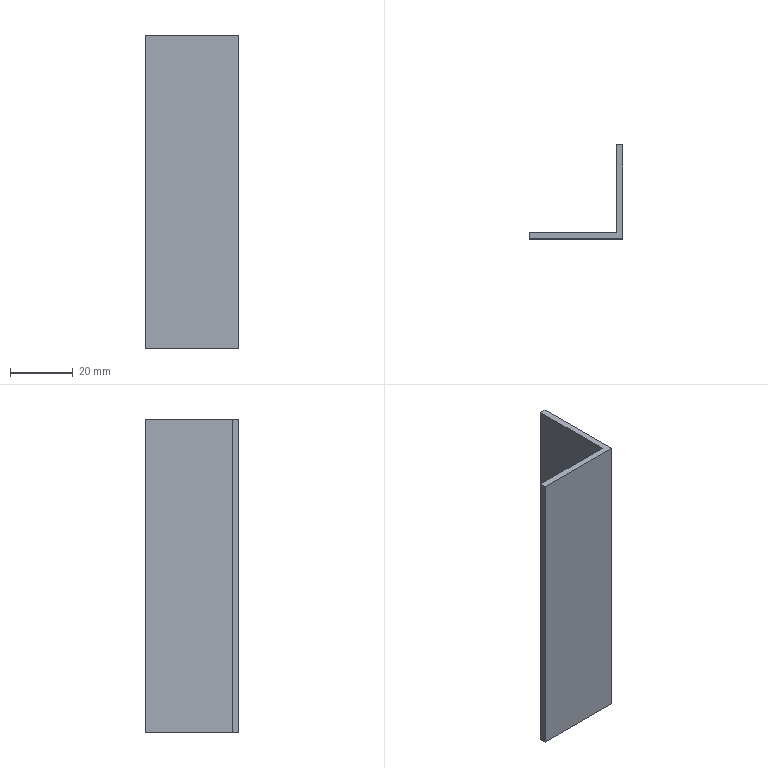Part | SolidWorks | features Extrusion 1 | 1 solid | 8 faces | box 30 x 30 x 100 mm | volume 11600 mm3 | plane 8
STEP:
#1=CARTESIAN_POINT('',(0.,2.,0.));
#2=VERTEX_POINT('',#1);
#3=CARTESIAN_POINT('',(0.,0.,0.));
#4=VERTEX_POINT('',#3);
#5=CARTESIAN_POINT('',(0.,0.,0.));
#6=DIRECTION('',(0.,-1.,0.));
#7=VECTOR('',#6,1000.);
#8=LINE('',#5,#7);
#9=EDGE_CURVE('',#2,#4,#8,.T.);
#10=ORIENTED_EDGE('',*,*,#9,.T.);
#11=CARTESIAN_POINT('',(0.,0.,100.));
#12=VERTEX_POINT('',#11);
#13=CARTESIAN_POINT('',(0.,0.,100.));
#14=DIRECTION('',(0.,0.,-1.));
#15=VECTOR('',#14,1000.);
#16=LINE('',#13,#15);
#17=EDGE_CURVE('',#12,#4,#16,.T.);
#18=ORIENTED_EDGE('',*,*,#17,.F.);
#19=CARTESIAN_POINT('',(0.,2.,100.));
#20=VERTEX_POINT('',#19);
#21=CARTESIAN_POINT('',(0.,0.,100.));
#22=DIRECTION('',(0.,-1.,0.));
#23=VECTOR('',#22,1000.);
#24=LINE('',#21,#23);
#25=EDGE_CURVE('',#20,#12,#24,.T.);
#26=ORIENTED_EDGE('',*,*,#25,.F.);
#27=CARTESIAN_POINT('',(0.,2.,100.));
#28=DIRECTION('',(0.,0.,-1.));
#29=VECTOR('',#28,1000.);
#30=LINE('',#27,#29);
#31=EDGE_CURVE('',#20,#2,#30,.T.);
#32=ORIENTED_EDGE('',*,*,#31,.T.);
#33=EDGE_LOOP('',(#10,#18,#26,#32));
#34=FACE_OUTER_BOUND('',#33,.T.);
#35=CARTESIAN_POINT('',(0.,0.,100.));
#36=DIRECTION('',(1.,0.,0.));
#37=DIRECTION('',(0.,0.,-1.));
#38=AXIS2_PLACEMENT_3D('',#35,#36,#37);
#39=PLANE('',#38);
#40=ADVANCED_FACE('',(#34),#39,.F.);
#41=CARTESIAN_POINT('',(30.,0.,0.));
#42=VERTEX_POINT('',#41);
#43=CARTESIAN_POINT('',(0.,0.,0.));
#44=DIRECTION('',(1.,0.,0.));
#45=VECTOR('',#44,1000.);
#46=LINE('',#43,#45);
#47=EDGE_CURVE('',#4,#42,#46,.T.);
#48=ORIENTED_EDGE('',*,*,#47,.T.);
#49=CARTESIAN_POINT('',(30.,0.,100.));
#50=VERTEX_POINT('',#49);
#51=CARTESIAN_POINT('',(30.,0.,100.));
#52=DIRECTION('',(0.,0.,-1.));
#53=VECTOR('',#52,1000.);
#54=LINE('',#51,#53);
#55=EDGE_CURVE('',#50,#42,#54,.T.);
#56=ORIENTED_EDGE('',*,*,#55,.F.);
#57=CARTESIAN_POINT('',(0.,0.,100.));
#58=DIRECTION('',(1.,0.,0.));
#59=VECTOR('',#58,1000.);
#60=LINE('',#57,#59);
#61=EDGE_CURVE('',#12,#50,#60,.T.);
#62=ORIENTED_EDGE('',*,*,#61,.F.);
#63=ORIENTED_EDGE('',*,*,#17,.T.);
#64=EDGE_LOOP('',(#48,#56,#62,#63));
#65=FACE_OUTER_BOUND('',#64,.T.);
#66=CARTESIAN_POINT('',(0.,0.,100.));
#67=DIRECTION('',(0.,1.,0.));
#68=DIRECTION('',(0.,0.,1.));
#69=AXIS2_PLACEMENT_3D('',#66,#67,#68);
#70=PLANE('',#69);
#71=ADVANCED_FACE('',(#65),#70,.F.);
#72=CARTESIAN_POINT('',(30.,30.,0.));
#73=VERTEX_POINT('',#72);
#74=CARTESIAN_POINT('',(30.,0.,0.));
#75=DIRECTION('',(0.,1.,0.));
#76=VECTOR('',#75,1000.);
#77=LINE('',#74,#76);
#78=EDGE_CURVE('',#42,#73,#77,.T.);
#79=ORIENTED_EDGE('',*,*,#78,.T.);
#80=CARTESIAN_POINT('',(30.,30.,100.));
#81=VERTEX_POINT('',#80);
#82=CARTESIAN_POINT('',(30.,30.,100.));
#83=DIRECTION('',(0.,0.,-1.));
#84=VECTOR('',#83,1000.);
#85=LINE('',#82,#84);
#86=EDGE_CURVE('',#81,#73,#85,.T.);
#87=ORIENTED_EDGE('',*,*,#86,.F.);
#88=CARTESIAN_POINT('',(30.,0.,100.));
#89=DIRECTION('',(0.,1.,0.));
#90=VECTOR('',#89,1000.);
#91=LINE('',#88,#90);
#92=EDGE_CURVE('',#50,#81,#91,.T.);
#93=ORIENTED_EDGE('',*,*,#92,.F.);
#94=ORIENTED_EDGE('',*,*,#55,.T.);
#95=EDGE_LOOP('',(#79,#87,#93,#94));
#96=FACE_OUTER_BOUND('',#95,.T.);
#97=CARTESIAN_POINT('',(30.,0.,100.));
#98=DIRECTION('',(-1.,0.,0.));
#99=DIRECTION('',(0.,0.,1.));
#100=AXIS2_PLACEMENT_3D('',#97,#98,#99);
#101=PLANE('',#100);
#102=ADVANCED_FACE('',(#96),#101,.F.);
#103=CARTESIAN_POINT('',(28.,30.,0.));
#104=VERTEX_POINT('',#103);
#105=CARTESIAN_POINT('',(28.,30.,0.));
#106=DIRECTION('',(-1.,0.,0.));
#107=VECTOR('',#106,1000.);
#108=LINE('',#105,#107);
#109=EDGE_CURVE('',#73,#104,#108,.T.);
#110=ORIENTED_EDGE('',*,*,#109,.T.);
#111=CARTESIAN_POINT('',(28.,30.,100.));
#112=VERTEX_POINT('',#111);
#113=CARTESIAN_POINT('',(28.,30.,100.));
#114=DIRECTION('',(0.,0.,-1.));
#115=VECTOR('',#114,1000.);
#116=LINE('',#113,#115);
#117=EDGE_CURVE('',#112,#104,#116,.T.);
#118=ORIENTED_EDGE('',*,*,#117,.F.);
#119=CARTESIAN_POINT('',(28.,30.,100.));
#120=DIRECTION('',(-1.,0.,0.));
#121=VECTOR('',#120,1000.);
#122=LINE('',#119,#121);
#123=EDGE_CURVE('',#81,#112,#122,.T.);
#124=ORIENTED_EDGE('',*,*,#123,.F.);
#125=ORIENTED_EDGE('',*,*,#86,.T.);
#126=EDGE_LOOP('',(#110,#118,#124,#125));
#127=FACE_OUTER_BOUND('',#126,.T.);
#128=CARTESIAN_POINT('',(28.,30.,100.));
#129=DIRECTION('',(0.,-1.,0.));
#130=DIRECTION('',(0.,0.,-1.));
#131=AXIS2_PLACEMENT_3D('',#128,#129,#130);
#132=PLANE('',#131);
#133=ADVANCED_FACE('',(#127),#132,.F.);
#134=CARTESIAN_POINT('',(28.,2.,0.));
#135=VERTEX_POINT('',#134);
#136=CARTESIAN_POINT('',(28.,2.,0.));
#137=DIRECTION('',(0.,-1.,0.));
#138=VECTOR('',#137,1000.);
#139=LINE('',#136,#138);
#140=EDGE_CURVE('',#104,#135,#139,.T.);
#141=ORIENTED_EDGE('',*,*,#140,.T.);
#142=CARTESIAN_POINT('',(28.,2.,100.));
#143=VERTEX_POINT('',#142);
#144=CARTESIAN_POINT('',(28.,2.,100.));
#145=DIRECTION('',(0.,0.,-1.));
#146=VECTOR('',#145,1000.);
#147=LINE('',#144,#146);
#148=EDGE_CURVE('',#143,#135,#147,.T.);
#149=ORIENTED_EDGE('',*,*,#148,.F.);
#150=CARTESIAN_POINT('',(28.,2.,100.));
#151=DIRECTION('',(0.,-1.,0.));
#152=VECTOR('',#151,1000.);
#153=LINE('',#150,#152);
#154=EDGE_CURVE('',#112,#143,#153,.T.);
#155=ORIENTED_EDGE('',*,*,#154,.F.);
#156=ORIENTED_EDGE('',*,*,#117,.T.);
#157=EDGE_LOOP('',(#141,#149,#155,#156));
#158=FACE_OUTER_BOUND('',#157,.T.);
#159=CARTESIAN_POINT('',(28.,2.,100.));
#160=DIRECTION('',(1.,0.,0.));
#161=DIRECTION('',(0.,0.,-1.));
#162=AXIS2_PLACEMENT_3D('',#159,#160,#161);
#163=PLANE('',#162);
#164=ADVANCED_FACE('',(#158),#163,.F.);
#165=CARTESIAN_POINT('',(0.,2.,0.));
#166=DIRECTION('',(-1.,0.,0.));
#167=VECTOR('',#166,1000.);
#168=LINE('',#165,#167);
#169=EDGE_CURVE('',#135,#2,#168,.T.);
#170=ORIENTED_EDGE('',*,*,#169,.T.);
#171=ORIENTED_EDGE('',*,*,#31,.F.);
#172=CARTESIAN_POINT('',(0.,2.,100.));
#173=DIRECTION('',(-1.,0.,0.));
#174=VECTOR('',#173,1000.);
#175=LINE('',#172,#174);
#176=EDGE_CURVE('',#143,#20,#175,.T.);
#177=ORIENTED_EDGE('',*,*,#176,.F.);
#178=ORIENTED_EDGE('',*,*,#148,.T.);
#179=EDGE_LOOP('',(#170,#171,#177,#178));
#180=FACE_OUTER_BOUND('',#179,.T.);
#181=CARTESIAN_POINT('',(0.,2.,100.));
#182=DIRECTION('',(0.,-1.,0.));
#183=DIRECTION('',(0.,0.,-1.));
#184=AXIS2_PLACEMENT_3D('',#181,#182,#183);
#185=PLANE('',#184);
#186=ADVANCED_FACE('',(#180),#185,.F.);
#187=ORIENTED_EDGE('',*,*,#25,.T.);
#188=ORIENTED_EDGE('',*,*,#61,.T.);
#189=ORIENTED_EDGE('',*,*,#92,.T.);
#190=ORIENTED_EDGE('',*,*,#123,.T.);
#191=ORIENTED_EDGE('',*,*,#154,.T.);
#192=ORIENTED_EDGE('',*,*,#176,.T.);
#193=EDGE_LOOP('',(#187,#188,#189,#190,#191,#192));
#194=FACE_OUTER_BOUND('',#193,.T.);
#195=CARTESIAN_POINT('',(0.,0.,100.));
#196=DIRECTION('',(0.,0.,-1.));
#197=DIRECTION('',(-1.,0.,0.));
#198=AXIS2_PLACEMENT_3D('',#195,#196,#197);
#199=PLANE('',#198);
#200=ADVANCED_FACE('',(#194),#199,.F.);
#201=ORIENTED_EDGE('',*,*,#9,.F.);
#202=ORIENTED_EDGE('',*,*,#169,.F.);
#203=ORIENTED_EDGE('',*,*,#140,.F.);
#204=ORIENTED_EDGE('',*,*,#109,.F.);
#205=ORIENTED_EDGE('',*,*,#78,.F.);
#206=ORIENTED_EDGE('',*,*,#47,.F.);
#207=EDGE_LOOP('',(#201,#202,#203,#204,#205,#206));
#208=FACE_OUTER_BOUND('',#207,.T.);
#209=CARTESIAN_POINT('',(0.,0.,0.));
#210=DIRECTION('',(0.,0.,-1.));
#211=DIRECTION('',(-1.,0.,0.));
#212=AXIS2_PLACEMENT_3D('',#209,#210,#211);
#213=PLANE('',#212);
#214=ADVANCED_FACE('',(#208),#213,.T.);
#215=CLOSED_SHELL('',(#40,#71,#102,#133,#164,#186,#200,#214));
#216=MANIFOLD_SOLID_BREP('',#215);
#217=CARTESIAN_POINT('',(0.,0.,0.));
#218=DIRECTION('',(0.,0.,1.));
#219=DIRECTION('',(1.,0.,0.));
#220=AXIS2_PLACEMENT_3D('',#217,#218,#219);
#221=(LENGTH_UNIT()NAMED_UNIT(*)SI_UNIT(.MILLI.,.METRE.));
#222=UNCERTAINTY_MEASURE_WITH_UNIT(LENGTH_MEASURE(0.00001),#221,'','');
#223=(NAMED_UNIT(*)PLANE_ANGLE_UNIT()SI_UNIT($,.RADIAN.));
#224=(NAMED_UNIT(*)SI_UNIT($,.STERADIAN.)SOLID_ANGLE_UNIT());
#225=(GEOMETRIC_REPRESENTATION_CONTEXT(3)GLOBAL_UNCERTAINTY_ASSIGNED_CONTEXT((#222))GLOBAL_UNIT_ASSIGNED_CONTEXT((#221,#223,#224))REPRESENTATION_CONTEXT('',''));
#226=ADVANCED_BREP_SHAPE_REPRESENTATION('',(#216,#220),#225);